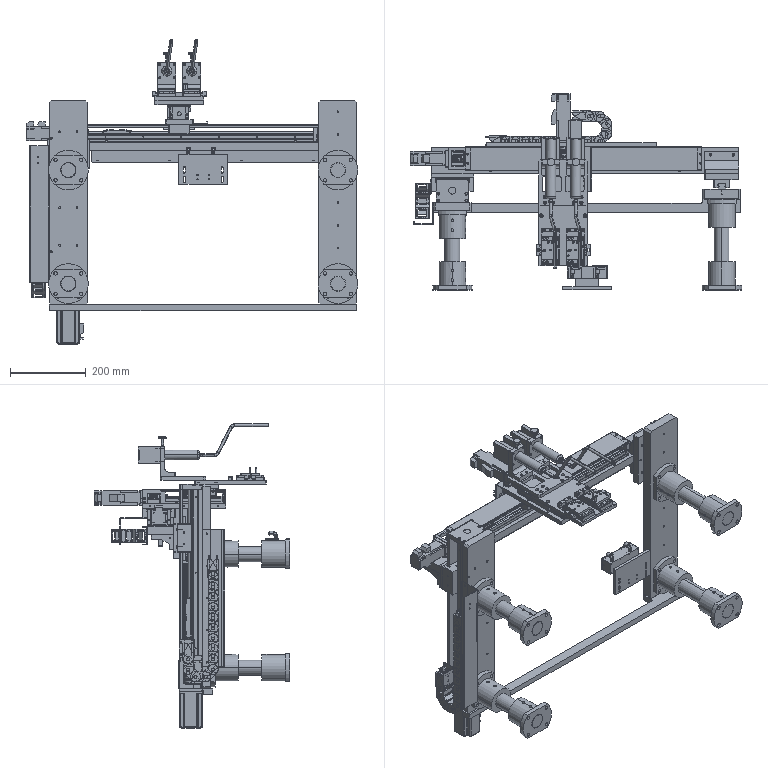Part | NX | features BREP 73 | 145 solids | 8244 faces | volume 12986994 mm3 | plane 4019 | cylinder 3418 | cone 607 | torus 130 | sphere 48 | spline 22 | commonest cylinder face diameters 8 x306 3.3 x232 4.5 x198 3 x176 5 x168 2.5 x162